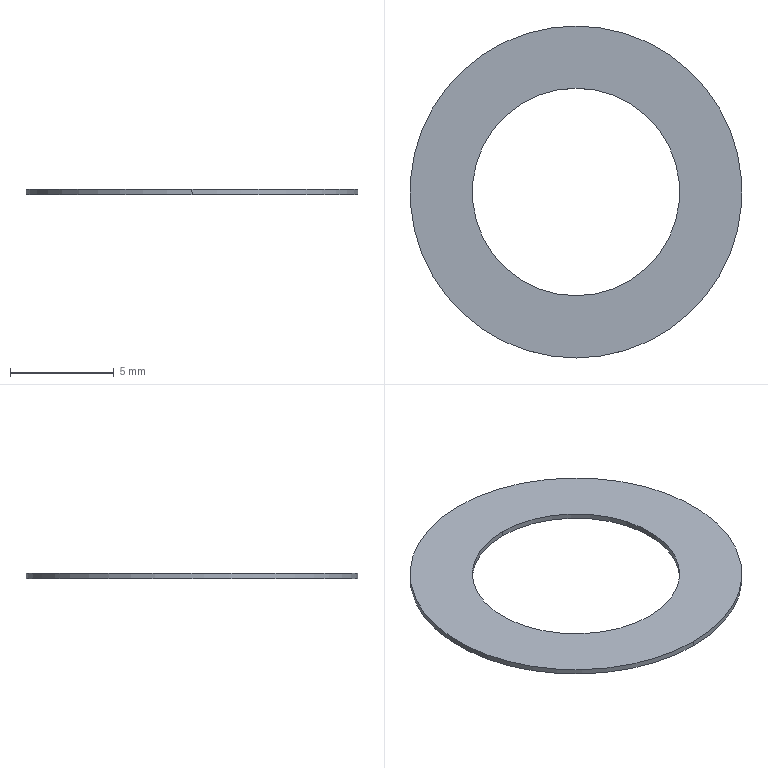Part | SolidWorks | features BaseBody 1 | 1 solid | 6 faces | box 16 x 16 x 0.25 mm | volume 30.631 mm3 | cylinder 4 | plane 2 | commonest cylinder face diameters 10 x2 16 x2
STEP:
#1=CARTESIAN_POINT('',(465.27,-106.215,305.544));
#2=VERTEX_POINT('',#1);
#3=CARTESIAN_POINT('',(465.27,-90.215,305.544));
#4=VERTEX_POINT('',#3);
#5=CARTESIAN_POINT('',(465.27,-98.215,305.544));
#6=DIRECTION('',(-0.000000001,-0.000000012,1.));
#7=DIRECTION('',(0.,-1.,-0.000000012));
#8=AXIS2_PLACEMENT_3D('',#5,#6,#7);
#9=CIRCLE('',#8,8.);
#10=EDGE_CURVE('',#2,#4,#9,.T.);
#11=ORIENTED_EDGE('',*,*,#10,.T.);
#12=CARTESIAN_POINT('',(465.27,-90.215,305.794));
#13=VERTEX_POINT('',#12);
#14=CARTESIAN_POINT('',(465.27,-90.215,305.794));
#15=DIRECTION('',(-0.000000001,-0.000000012,1.));
#16=VECTOR('',#15,1000.);
#17=LINE('',#14,#16);
#18=EDGE_CURVE('',#4,#13,#17,.T.);
#19=ORIENTED_EDGE('',*,*,#18,.T.);
#20=CARTESIAN_POINT('',(465.27,-106.215,305.794));
#21=VERTEX_POINT('',#20);
#22=CARTESIAN_POINT('',(465.27,-98.215,305.794));
#23=DIRECTION('',(0.000000001,0.000000012,-1.));
#24=DIRECTION('',(0.,-1.,-0.000000012));
#25=AXIS2_PLACEMENT_3D('',#22,#23,#24);
#26=CIRCLE('',#25,8.);
#27=EDGE_CURVE('',#13,#21,#26,.T.);
#28=ORIENTED_EDGE('',*,*,#27,.T.);
#29=CARTESIAN_POINT('',(465.27,-106.215,305.794));
#30=DIRECTION('',(-0.000000001,-0.000000012,1.));
#31=VECTOR('',#30,1000.);
#32=LINE('',#29,#31);
#33=EDGE_CURVE('',#2,#21,#32,.T.);
#34=ORIENTED_EDGE('',*,*,#33,.F.);
#35=EDGE_LOOP('',(#11,#19,#28,#34));
#36=FACE_OUTER_BOUND('',#35,.T.);
#37=CARTESIAN_POINT('',(465.27,-98.215,305.794));
#38=DIRECTION('',(-0.000000001,-0.000000012,1.));
#39=DIRECTION('',(0.,-1.,-0.000000012));
#40=AXIS2_PLACEMENT_3D('',#37,#38,#39);
#41=CYLINDRICAL_SURFACE('',#40,8.);
#42=ADVANCED_FACE('',(#36),#41,.T.);
#43=CARTESIAN_POINT('',(465.27,-93.215,305.544));
#44=VERTEX_POINT('',#43);
#45=CARTESIAN_POINT('',(465.27,-103.215,305.544));
#46=VERTEX_POINT('',#45);
#47=CARTESIAN_POINT('',(465.27,-98.215,305.544));
#48=DIRECTION('',(-0.000000001,-0.000000012,1.));
#49=DIRECTION('',(0.,-1.,-0.000000012));
#50=AXIS2_PLACEMENT_3D('',#47,#48,#49);
#51=CIRCLE('',#50,5.);
#52=EDGE_CURVE('',#44,#46,#51,.T.);
#53=ORIENTED_EDGE('',*,*,#52,.F.);
#54=CARTESIAN_POINT('',(465.27,-93.215,305.794));
#55=VERTEX_POINT('',#54);
#56=CARTESIAN_POINT('',(465.27,-93.215,305.794));
#57=DIRECTION('',(-0.000000001,-0.000000012,1.));
#58=VECTOR('',#57,1000.);
#59=LINE('',#56,#58);
#60=EDGE_CURVE('',#44,#55,#59,.T.);
#61=ORIENTED_EDGE('',*,*,#60,.T.);
#62=CARTESIAN_POINT('',(465.27,-103.215,305.794));
#63=VERTEX_POINT('',#62);
#64=CARTESIAN_POINT('',(465.27,-98.215,305.794));
#65=DIRECTION('',(-0.000000001,-0.000000012,1.));
#66=DIRECTION('',(0.,-1.,-0.000000012));
#67=AXIS2_PLACEMENT_3D('',#64,#65,#66);
#68=CIRCLE('',#67,5.);
#69=EDGE_CURVE('',#55,#63,#68,.T.);
#70=ORIENTED_EDGE('',*,*,#69,.T.);
#71=CARTESIAN_POINT('',(465.27,-103.215,305.794));
#72=DIRECTION('',(-0.000000001,-0.000000012,1.));
#73=VECTOR('',#72,1000.);
#74=LINE('',#71,#73);
#75=EDGE_CURVE('',#46,#63,#74,.T.);
#76=ORIENTED_EDGE('',*,*,#75,.F.);
#77=EDGE_LOOP('',(#53,#61,#70,#76));
#78=FACE_OUTER_BOUND('',#77,.T.);
#79=CARTESIAN_POINT('',(465.27,-98.215,305.794));
#80=DIRECTION('',(-0.000000001,-0.000000012,1.));
#81=DIRECTION('',(0.,-1.,-0.000000012));
#82=AXIS2_PLACEMENT_3D('',#79,#80,#81);
#83=CYLINDRICAL_SURFACE('',#82,5.);
#84=ADVANCED_FACE('',(#78),#83,.F.);
#85=CARTESIAN_POINT('',(465.27,-98.215,305.794));
#86=DIRECTION('',(0.000000001,0.000000012,-1.));
#87=DIRECTION('',(0.,-1.,-0.000000012));
#88=AXIS2_PLACEMENT_3D('',#85,#86,#87);
#89=CIRCLE('',#88,8.);
#90=EDGE_CURVE('',#21,#13,#89,.T.);
#91=ORIENTED_EDGE('',*,*,#90,.F.);
#92=ORIENTED_EDGE('',*,*,#27,.F.);
#93=EDGE_LOOP('',(#91,#92));
#94=FACE_OUTER_BOUND('',#93,.T.);
#95=CARTESIAN_POINT('',(465.27,-98.215,305.794));
#96=DIRECTION('',(-0.000000001,-0.000000012,1.));
#97=DIRECTION('',(0.,-1.,-0.000000012));
#98=AXIS2_PLACEMENT_3D('',#95,#96,#97);
#99=CIRCLE('',#98,5.);
#100=EDGE_CURVE('',#63,#55,#99,.T.);
#101=ORIENTED_EDGE('',*,*,#100,.F.);
#102=ORIENTED_EDGE('',*,*,#69,.F.);
#103=EDGE_LOOP('',(#101,#102));
#104=FACE_BOUND('',#103,.T.);
#105=CARTESIAN_POINT('',(465.27,-98.215,305.794));
#106=DIRECTION('',(0.000000001,0.000000012,-1.));
#107=DIRECTION('',(0.,1.,0.000000012));
#108=AXIS2_PLACEMENT_3D('',#105,#106,#107);
#109=PLANE('',#108);
#110=ADVANCED_FACE('',(#94,#104),#109,.F.);
#111=ORIENTED_EDGE('',*,*,#18,.F.);
#112=CARTESIAN_POINT('',(465.27,-98.215,305.544));
#113=DIRECTION('',(-0.000000001,-0.000000012,1.));
#114=DIRECTION('',(0.,-1.,-0.000000012));
#115=AXIS2_PLACEMENT_3D('',#112,#113,#114);
#116=CIRCLE('',#115,8.);
#117=EDGE_CURVE('',#4,#2,#116,.T.);
#118=ORIENTED_EDGE('',*,*,#117,.T.);
#119=ORIENTED_EDGE('',*,*,#33,.T.);
#120=ORIENTED_EDGE('',*,*,#90,.T.);
#121=EDGE_LOOP('',(#111,#118,#119,#120));
#122=FACE_OUTER_BOUND('',#121,.T.);
#123=CARTESIAN_POINT('',(465.27,-98.215,305.794));
#124=DIRECTION('',(-0.000000001,-0.000000012,1.));
#125=DIRECTION('',(0.,-1.,-0.000000012));
#126=AXIS2_PLACEMENT_3D('',#123,#124,#125);
#127=CYLINDRICAL_SURFACE('',#126,8.);
#128=ADVANCED_FACE('',(#122),#127,.T.);
#129=ORIENTED_EDGE('',*,*,#60,.F.);
#130=CARTESIAN_POINT('',(465.27,-98.215,305.544));
#131=DIRECTION('',(-0.000000001,-0.000000012,1.));
#132=DIRECTION('',(0.,-1.,-0.000000012));
#133=AXIS2_PLACEMENT_3D('',#130,#131,#132);
#134=CIRCLE('',#133,5.);
#135=EDGE_CURVE('',#46,#44,#134,.T.);
#136=ORIENTED_EDGE('',*,*,#135,.F.);
#137=ORIENTED_EDGE('',*,*,#75,.T.);
#138=ORIENTED_EDGE('',*,*,#100,.T.);
#139=EDGE_LOOP('',(#129,#136,#137,#138));
#140=FACE_OUTER_BOUND('',#139,.T.);
#141=CARTESIAN_POINT('',(465.27,-98.215,305.794));
#142=DIRECTION('',(-0.000000001,-0.000000012,1.));
#143=DIRECTION('',(0.,-1.,-0.000000012));
#144=AXIS2_PLACEMENT_3D('',#141,#142,#143);
#145=CYLINDRICAL_SURFACE('',#144,5.);
#146=ADVANCED_FACE('',(#140),#145,.F.);
#147=ORIENTED_EDGE('',*,*,#10,.F.);
#148=ORIENTED_EDGE('',*,*,#117,.F.);
#149=EDGE_LOOP('',(#147,#148));
#150=FACE_OUTER_BOUND('',#149,.T.);
#151=ORIENTED_EDGE('',*,*,#135,.T.);
#152=ORIENTED_EDGE('',*,*,#52,.T.);
#153=EDGE_LOOP('',(#151,#152));
#154=FACE_BOUND('',#153,.T.);
#155=CARTESIAN_POINT('',(465.27,-98.215,305.544));
#156=DIRECTION('',(0.000000001,0.000000012,-1.));
#157=DIRECTION('',(0.,1.,0.000000012));
#158=AXIS2_PLACEMENT_3D('',#155,#156,#157);
#159=PLANE('',#158);
#160=ADVANCED_FACE('',(#150,#154),#159,.T.);
#161=CLOSED_SHELL('',(#42,#84,#110,#128,#146,#160));
#162=MANIFOLD_SOLID_BREP('',#161);
#163=CARTESIAN_POINT('',(0.,0.,0.));
#164=DIRECTION('',(0.,0.,1.));
#165=DIRECTION('',(1.,0.,0.));
#166=AXIS2_PLACEMENT_3D('',#163,#164,#165);
#167=(LENGTH_UNIT()NAMED_UNIT(*)SI_UNIT(.MILLI.,.METRE.));
#168=UNCERTAINTY_MEASURE_WITH_UNIT(LENGTH_MEASURE(0.00001),#167,'','');
#169=(NAMED_UNIT(*)PLANE_ANGLE_UNIT()SI_UNIT($,.RADIAN.));
#170=(NAMED_UNIT(*)SI_UNIT($,.STERADIAN.)SOLID_ANGLE_UNIT());
#171=(GEOMETRIC_REPRESENTATION_CONTEXT(3)GLOBAL_UNCERTAINTY_ASSIGNED_CONTEXT((#168))GLOBAL_UNIT_ASSIGNED_CONTEXT((#167,#169,#170))REPRESENTATION_CONTEXT('',''));
#172=ADVANCED_BREP_SHAPE_REPRESENTATION('',(#162,#166),#171);